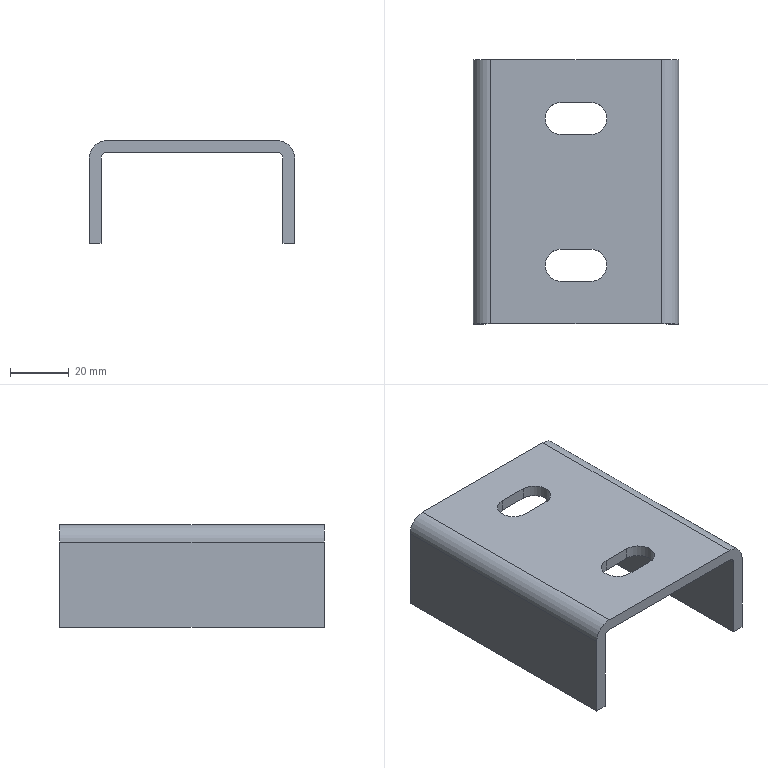Part | STEP file | HL4GZ-1.581.109 (auxiliary valve bracket fixing seat) | 1 solid | 22 faces | box 70 x 90 x 35 mm | volume 44644 mm3 | plane 14 | cylinder 8 | commonest cylinder face diameters 11 x4 4 x2 12 x2